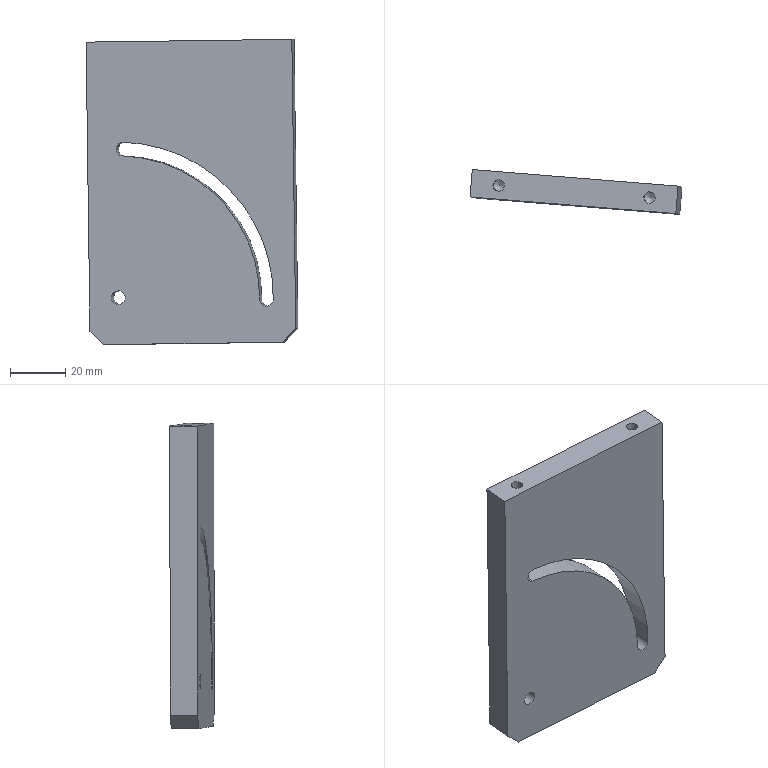CAM job | NX | 3+2 milling, drilling | part box 76.959 x 16.139 x 110.936 mm | stock box 82.237 x 18.548 x 116.071 mm
Tools:
number,name,description,diameter,corner_radius,flute_length,length,flutes
4,D4,平底铣刀-粗,4.0,0.0,25.0,75.0,2
9,D10,平底铣刀-粗,10.0,0.0,35.0,75.0,2
11,D4-J,平底铣刀-精,4.0,0.0,50.0,75.0,2
10,D10-J,平底铣刀-精,10.0,0.0,35.0,75.0,2
1,D80R0.8飞刀,圆鼻刀-粗,80.0,0.8,50.0,75.0,2
1,D80R0.8飞刀-J,圆鼻刀-精,80.0,0.8,50.0,75.0,2
2,D6倒角刀,倒角刀,6.0,0.0,3.0,25.0,2
18,D5铰刀,Drilling Tool,5.0,0.0,75.0,100.0,6
17,ZT4.9,Drilling Tool,4.9,0.0,35.0,50.0,2
Operations:
program,operation,operation_type,tool,method,geometry_group,spindle_rpm,surface_speed,feed_per_tooth,feed_cut,feed_plunge,cut_length_mm,path_length_mm,cut_time_min,machine_time_min
B,BOTTOMWALL_FLYFACEROUGH_COPY,VolumeBased25DMillingOperation,D80R0.8飞刀,LAYER-ROUGH-DEPTHK-STEPG,W-B,2800.0,703.696,0.5357,3000.0,100.0,872.776,1549.735,0.2909,0.3586
B,BOTTOMWALL_FLYFACEFINISH_COPY,VolumeBased25DMillingOperation,D80R0.8飞刀-J,SIDEFINISH-DEPTHK-STEPG,W-B,4000.0,1005.28,0.125,1000.0,100.0,217.998,253.998,0.218,0.2216
B,PLANARDEBURR6X45L_COPY,SurfaceContour,D6倒角刀,CLIMBCHAMFER-DEPTH0-STEPG,W-B,6500.0,122.519,0.1154,1500.0,100.0,567.693,728.032,0.3785,0.3945
A,TOPFACE,FaceMilling,D80R0.8飞刀,SIDEFINISH-DEPTHK-STEPG,W-A,4000.0,1005.31,0.125,1000.0,100.0,445.667,481.667,0.4457,0.4493
A,PROFILE_ROUGH_2,VolumeBased25DMillingOperation,D10,METHOD,W-A,8000.0,251.327,0.3125,5000.0,80.0,5944.306,5992.806,1.189,1.194
A,SPOTDRILL-DEPTH0.8,Operation,D6倒角刀,NONE,W-A,8000.0,150.796,0.0312,500.0,90.0,5.4,182.32,0.0108,0.0285
A,THRUHOLE-PILOT6.0,Operation,ZT4.9,NONE,W-A,2500.0,38.484,0.05,250.0,90.0,46.243,264.007,0.185,0.2068
A,BOTTOMWALL_SPIRALROUGH-SMALL_COPY,VolumeBased25DMillingOperation,D4,LAYER-ROUGH-DEPTHK-STEPG,W-A,8000.0,100.528,0.125,2000.0,100.0,6126.823,6175.423,3.063,3.068
A,SELECTBODYONLY,SurfaceContour,D6倒角刀,METHOD,W-A,8000.0,150.796,0.1875,3000.0,100.0,565.369,689.677,0.1885,0.2009
A,MILLCHAMFER_1,PlanarMilling,D6倒角刀,METHOD,W-A,8000.0,150.796,0.0312,500.0,100.0,18.482,59.481,0.037,0.0411
A,REAM,Operation,D5铰刀,METHOD,W-A,500.0,7.854,0.0167,50.0,0.0,12.0,64.0,0.24,0.2452
A,BOTTOMWALL_SPIRALFINISH-SMALL_COPY,VolumeBased25DMillingOperation,D4-J,SPIRALFINISH-DEPTHK-STEPG,W-A,8000.0,100.528,0.05,800.0,100.0,1203.701,1252.401,1.505,1.51
A,PROFILE_SEMIFINISH_2,VolumeBased25DMillingOperation,D10-J,METHOD,W-A,8000.0,251.327,0.0625,1000.0,100.0,400.516,459.516,0.4005,0.4064